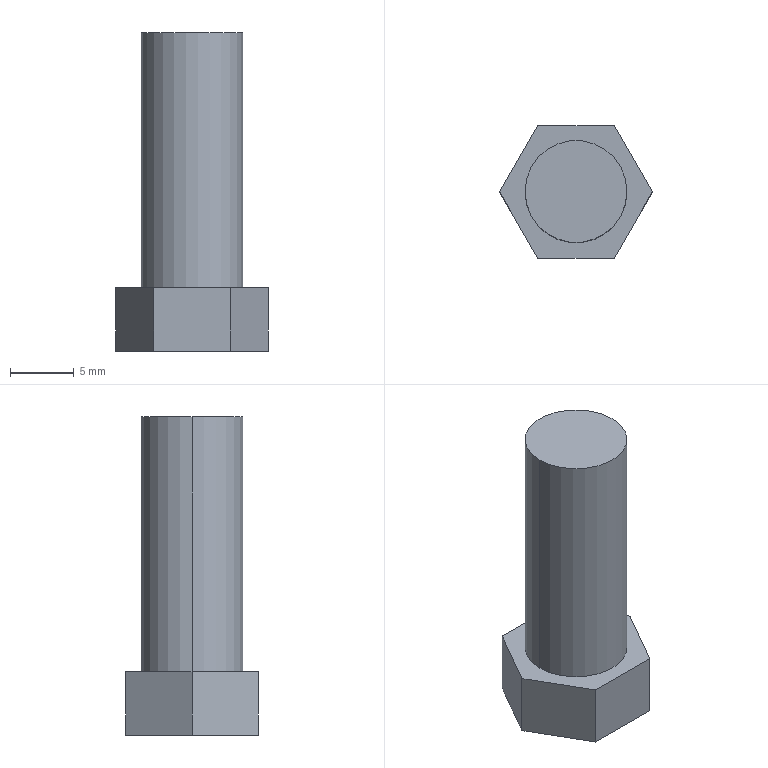Part | NX | features BREP 1, DATUM_CSYS 1, EXTRUDE 1, SKETCH 1 | 1 solid | 18 faces | box 12 x 10.392 x 25 mm | volume 1379 mm3 | plane 16 | cylinder 2 | commonest cylinder face diameters 8 x2
STEP:
#1=CARTESIAN_POINT('',(4.,0.,25.));
#2=VERTEX_POINT('',#1);
#3=CARTESIAN_POINT('',(-4.,0.,25.));
#4=VERTEX_POINT('',#3);
#5=CARTESIAN_POINT('',(0.,0.,25.));
#6=DIRECTION('',(0.,0.,1.));
#7=DIRECTION('',(1.,0.,0.));
#8=AXIS2_PLACEMENT_3D('',#5,#6,#7);
#9=CIRCLE('',#8,4.);
#10=EDGE_CURVE('',#2,#4,#9,.T.);
#11=ORIENTED_EDGE('',*,*,#10,.F.);
#12=CARTESIAN_POINT('',(4.,0.,5.));
#13=VERTEX_POINT('',#12);
#14=CARTESIAN_POINT('',(4.,0.,10.));
#15=DIRECTION('',(0.,0.,-1.));
#16=VECTOR('',#15,1000.);
#17=LINE('',#14,#16);
#18=EDGE_CURVE('',#13,#2,#17,.F.);
#19=ORIENTED_EDGE('',*,*,#18,.F.);
#20=CARTESIAN_POINT('',(-4.,0.,5.));
#21=VERTEX_POINT('',#20);
#22=CARTESIAN_POINT('',(0.,0.,5.));
#23=DIRECTION('',(0.,0.,1.));
#24=DIRECTION('',(1.,0.,0.));
#25=AXIS2_PLACEMENT_3D('',#22,#23,#24);
#26=CIRCLE('',#25,4.);
#27=EDGE_CURVE('',#13,#21,#26,.T.);
#28=ORIENTED_EDGE('',*,*,#27,.T.);
#29=CARTESIAN_POINT('',(-4.,0.,10.));
#30=DIRECTION('',(0.,0.,-1.));
#31=VECTOR('',#30,1000.);
#32=LINE('',#29,#31);
#33=EDGE_CURVE('',#21,#4,#32,.F.);
#34=ORIENTED_EDGE('',*,*,#33,.T.);
#35=EDGE_LOOP('',(#11,#19,#28,#34));
#36=FACE_BOUND('',#35,.T.);
#37=CARTESIAN_POINT('',(0.,0.,10.));
#38=DIRECTION('',(0.,0.,-1.));
#39=DIRECTION('',(1.,0.,0.));
#40=AXIS2_PLACEMENT_3D('',#37,#38,#39);
#41=CYLINDRICAL_SURFACE('',#40,4.);
#42=ADVANCED_FACE('',(#36),#41,.T.);
#43=CARTESIAN_POINT('',(3.,5.196,0.));
#44=VERTEX_POINT('',#43);
#45=CARTESIAN_POINT('',(-3.,5.196,0.));
#46=VERTEX_POINT('',#45);
#47=CARTESIAN_POINT('',(0.,5.196,0.));
#48=DIRECTION('',(-1.,0.,0.));
#49=VECTOR('',#48,1000.);
#50=LINE('',#47,#49);
#51=EDGE_CURVE('',#44,#46,#50,.T.);
#52=ORIENTED_EDGE('',*,*,#51,.T.);
#53=CARTESIAN_POINT('',(-3.,5.196,5.));
#54=VERTEX_POINT('',#53);
#55=CARTESIAN_POINT('',(-3.,5.196,5.));
#56=DIRECTION('',(0.,0.,-1.));
#57=VECTOR('',#56,1000.);
#58=LINE('',#55,#57);
#59=EDGE_CURVE('',#54,#46,#58,.T.);
#60=ORIENTED_EDGE('',*,*,#59,.F.);
#61=CARTESIAN_POINT('',(3.,5.196,5.));
#62=VERTEX_POINT('',#61);
#63=CARTESIAN_POINT('',(0.,5.196,5.));
#64=DIRECTION('',(-1.,0.,0.));
#65=VECTOR('',#64,1000.);
#66=LINE('',#63,#65);
#67=EDGE_CURVE('',#62,#54,#66,.T.);
#68=ORIENTED_EDGE('',*,*,#67,.F.);
#69=CARTESIAN_POINT('',(3.,5.196,5.));
#70=DIRECTION('',(0.,0.,-1.));
#71=VECTOR('',#70,1000.);
#72=LINE('',#69,#71);
#73=EDGE_CURVE('',#62,#44,#72,.T.);
#74=ORIENTED_EDGE('',*,*,#73,.T.);
#75=EDGE_LOOP('',(#52,#60,#68,#74));
#76=FACE_BOUND('',#75,.T.);
#77=CARTESIAN_POINT('',(0.,5.196,5.));
#78=DIRECTION('',(0.,-1.,0.));
#79=DIRECTION('',(-1.,0.,0.));
#80=AXIS2_PLACEMENT_3D('',#77,#78,#79);
#81=PLANE('',#80);
#82=ADVANCED_FACE('',(#76),#81,.F.);
#83=CARTESIAN_POINT('',(-6.,0.,0.));
#84=VERTEX_POINT('',#83);
#85=CARTESIAN_POINT('',(-4.5,2.598,0.));
#86=DIRECTION('',(-0.5,-0.866,0.));
#87=VECTOR('',#86,1000.);
#88=LINE('',#85,#87);
#89=EDGE_CURVE('',#46,#84,#88,.T.);
#90=ORIENTED_EDGE('',*,*,#89,.T.);
#91=CARTESIAN_POINT('',(-6.,0.,5.));
#92=VERTEX_POINT('',#91);
#93=CARTESIAN_POINT('',(-6.,0.,5.));
#94=DIRECTION('',(0.,0.,-1.));
#95=VECTOR('',#94,1000.);
#96=LINE('',#93,#95);
#97=EDGE_CURVE('',#92,#84,#96,.T.);
#98=ORIENTED_EDGE('',*,*,#97,.F.);
#99=CARTESIAN_POINT('',(-4.5,2.598,5.));
#100=DIRECTION('',(-0.5,-0.866,0.));
#101=VECTOR('',#100,1000.);
#102=LINE('',#99,#101);
#103=EDGE_CURVE('',#54,#92,#102,.T.);
#104=ORIENTED_EDGE('',*,*,#103,.F.);
#105=ORIENTED_EDGE('',*,*,#59,.T.);
#106=EDGE_LOOP('',(#90,#98,#104,#105));
#107=FACE_BOUND('',#106,.T.);
#108=CARTESIAN_POINT('',(-4.5,2.598,5.));
#109=DIRECTION('',(0.866,-0.5,0.));
#110=DIRECTION('',(-0.5,-0.866,0.));
#111=AXIS2_PLACEMENT_3D('',#108,#109,#110);
#112=PLANE('',#111);
#113=ADVANCED_FACE('',(#107),#112,.F.);
#114=CARTESIAN_POINT('',(-3.,-5.196,0.));
#115=VERTEX_POINT('',#114);
#116=CARTESIAN_POINT('',(-4.5,-2.598,0.));
#117=DIRECTION('',(0.5,-0.866,0.));
#118=VECTOR('',#117,1000.);
#119=LINE('',#116,#118);
#120=EDGE_CURVE('',#84,#115,#119,.T.);
#121=ORIENTED_EDGE('',*,*,#120,.T.);
#122=CARTESIAN_POINT('',(-3.,-5.196,5.));
#123=VERTEX_POINT('',#122);
#124=CARTESIAN_POINT('',(-3.,-5.196,5.));
#125=DIRECTION('',(0.,0.,-1.));
#126=VECTOR('',#125,1000.);
#127=LINE('',#124,#126);
#128=EDGE_CURVE('',#123,#115,#127,.T.);
#129=ORIENTED_EDGE('',*,*,#128,.F.);
#130=CARTESIAN_POINT('',(-4.5,-2.598,5.));
#131=DIRECTION('',(0.5,-0.866,0.));
#132=VECTOR('',#131,1000.);
#133=LINE('',#130,#132);
#134=EDGE_CURVE('',#92,#123,#133,.T.);
#135=ORIENTED_EDGE('',*,*,#134,.F.);
#136=ORIENTED_EDGE('',*,*,#97,.T.);
#137=EDGE_LOOP('',(#121,#129,#135,#136));
#138=FACE_BOUND('',#137,.T.);
#139=CARTESIAN_POINT('',(-4.5,-2.598,5.));
#140=DIRECTION('',(0.866,0.5,0.));
#141=DIRECTION('',(0.5,-0.866,0.));
#142=AXIS2_PLACEMENT_3D('',#139,#140,#141);
#143=PLANE('',#142);
#144=ADVANCED_FACE('',(#138),#143,.F.);
#145=CARTESIAN_POINT('',(3.,-5.196,0.));
#146=VERTEX_POINT('',#145);
#147=CARTESIAN_POINT('',(0.,-5.196,0.));
#148=DIRECTION('',(1.,0.,0.));
#149=VECTOR('',#148,1000.);
#150=LINE('',#147,#149);
#151=EDGE_CURVE('',#115,#146,#150,.T.);
#152=ORIENTED_EDGE('',*,*,#151,.T.);
#153=CARTESIAN_POINT('',(3.,-5.196,5.));
#154=VERTEX_POINT('',#153);
#155=CARTESIAN_POINT('',(3.,-5.196,5.));
#156=DIRECTION('',(0.,0.,-1.));
#157=VECTOR('',#156,1000.);
#158=LINE('',#155,#157);
#159=EDGE_CURVE('',#154,#146,#158,.T.);
#160=ORIENTED_EDGE('',*,*,#159,.F.);
#161=CARTESIAN_POINT('',(0.,-5.196,5.));
#162=DIRECTION('',(1.,0.,0.));
#163=VECTOR('',#162,1000.);
#164=LINE('',#161,#163);
#165=EDGE_CURVE('',#123,#154,#164,.T.);
#166=ORIENTED_EDGE('',*,*,#165,.F.);
#167=ORIENTED_EDGE('',*,*,#128,.T.);
#168=EDGE_LOOP('',(#152,#160,#166,#167));
#169=FACE_BOUND('',#168,.T.);
#170=CARTESIAN_POINT('',(0.,-5.196,5.));
#171=DIRECTION('',(0.,1.,0.));
#172=DIRECTION('',(1.,0.,0.));
#173=AXIS2_PLACEMENT_3D('',#170,#171,#172);
#174=PLANE('',#173);
#175=ADVANCED_FACE('',(#169),#174,.F.);
#176=CARTESIAN_POINT('',(6.,0.,0.));
#177=VERTEX_POINT('',#176);
#178=CARTESIAN_POINT('',(4.5,-2.598,0.));
#179=DIRECTION('',(0.5,0.866,0.));
#180=VECTOR('',#179,1000.);
#181=LINE('',#178,#180);
#182=EDGE_CURVE('',#146,#177,#181,.T.);
#183=ORIENTED_EDGE('',*,*,#182,.T.);
#184=CARTESIAN_POINT('',(6.,0.,5.));
#185=VERTEX_POINT('',#184);
#186=CARTESIAN_POINT('',(6.,0.,5.));
#187=DIRECTION('',(0.,0.,-1.));
#188=VECTOR('',#187,1000.);
#189=LINE('',#186,#188);
#190=EDGE_CURVE('',#185,#177,#189,.T.);
#191=ORIENTED_EDGE('',*,*,#190,.F.);
#192=CARTESIAN_POINT('',(4.5,-2.598,5.));
#193=DIRECTION('',(0.5,0.866,0.));
#194=VECTOR('',#193,1000.);
#195=LINE('',#192,#194);
#196=EDGE_CURVE('',#154,#185,#195,.T.);
#197=ORIENTED_EDGE('',*,*,#196,.F.);
#198=ORIENTED_EDGE('',*,*,#159,.T.);
#199=EDGE_LOOP('',(#183,#191,#197,#198));
#200=FACE_BOUND('',#199,.T.);
#201=CARTESIAN_POINT('',(4.5,-2.598,5.));
#202=DIRECTION('',(-0.866,0.5,0.));
#203=DIRECTION('',(0.5,0.866,0.));
#204=AXIS2_PLACEMENT_3D('',#201,#202,#203);
#205=PLANE('',#204);
#206=ADVANCED_FACE('',(#200),#205,.F.);
#207=CARTESIAN_POINT('',(4.5,2.598,0.));
#208=DIRECTION('',(-0.5,0.866,0.));
#209=VECTOR('',#208,1000.);
#210=LINE('',#207,#209);
#211=EDGE_CURVE('',#177,#44,#210,.T.);
#212=ORIENTED_EDGE('',*,*,#211,.T.);
#213=ORIENTED_EDGE('',*,*,#73,.F.);
#214=CARTESIAN_POINT('',(4.5,2.598,5.));
#215=DIRECTION('',(-0.5,0.866,0.));
#216=VECTOR('',#215,1000.);
#217=LINE('',#214,#216);
#218=EDGE_CURVE('',#185,#62,#217,.T.);
#219=ORIENTED_EDGE('',*,*,#218,.F.);
#220=ORIENTED_EDGE('',*,*,#190,.T.);
#221=EDGE_LOOP('',(#212,#213,#219,#220));
#222=FACE_BOUND('',#221,.T.);
#223=CARTESIAN_POINT('',(4.5,2.598,5.));
#224=DIRECTION('',(-0.866,-0.5,0.));
#225=DIRECTION('',(-0.5,0.866,0.));
#226=AXIS2_PLACEMENT_3D('',#223,#224,#225);
#227=PLANE('',#226);
#228=ADVANCED_FACE('',(#222),#227,.F.);
#229=CARTESIAN_POINT('',(0.,0.,5.));
#230=DIRECTION('',(0.,0.,1.));
#231=DIRECTION('',(1.,0.,0.));
#232=AXIS2_PLACEMENT_3D('',#229,#230,#231);
#233=CIRCLE('',#232,4.);
#234=EDGE_CURVE('',#21,#13,#233,.T.);
#235=ORIENTED_EDGE('',*,*,#234,.F.);
#236=ORIENTED_EDGE('',*,*,#27,.F.);
#237=EDGE_LOOP('',(#235,#236));
#238=FACE_BOUND('',#237,.T.);
#239=ORIENTED_EDGE('',*,*,#67,.T.);
#240=ORIENTED_EDGE('',*,*,#103,.T.);
#241=ORIENTED_EDGE('',*,*,#134,.T.);
#242=ORIENTED_EDGE('',*,*,#165,.T.);
#243=ORIENTED_EDGE('',*,*,#196,.T.);
#244=ORIENTED_EDGE('',*,*,#218,.T.);
#245=EDGE_LOOP('',(#239,#240,#241,#242,#243,#244));
#246=FACE_BOUND('',#245,.T.);
#247=CARTESIAN_POINT('',(0.,0.,5.));
#248=DIRECTION('',(0.,0.,1.));
#249=DIRECTION('',(-1.,0.,0.));
#250=AXIS2_PLACEMENT_3D('',#247,#248,#249);
#251=PLANE('',#250);
#252=ADVANCED_FACE('',(#238,#246),#251,.T.);
#253=CARTESIAN_POINT('',(-2.085,-2.767,0.));
#254=VERTEX_POINT('',#253);
#255=CARTESIAN_POINT('',(-3.438,0.4222,0.));
#256=VERTEX_POINT('',#255);
#257=CARTESIAN_POINT('',(-2.085,-2.767,0.));
#258=DIRECTION('',(-0.3907,0.9205,0.));
#259=VECTOR('',#258,1000.);
#260=LINE('',#257,#259);
#261=EDGE_CURVE('',#254,#256,#260,.T.);
#262=ORIENTED_EDGE('',*,*,#261,.F.);
#263=CARTESIAN_POINT('',(1.354,-3.189,0.));
#264=VERTEX_POINT('',#263);
#265=CARTESIAN_POINT('',(1.354,-3.189,0.));
#266=DIRECTION('',(-0.9925,0.1219,0.));
#267=VECTOR('',#266,1000.);
#268=LINE('',#265,#267);
#269=EDGE_CURVE('',#264,#254,#268,.T.);
#270=ORIENTED_EDGE('',*,*,#269,.F.);
#271=CARTESIAN_POINT('',(3.438,-0.4222,0.));
#272=VERTEX_POINT('',#271);
#273=CARTESIAN_POINT('',(3.438,-0.4222,0.));
#274=DIRECTION('',(-0.6018,-0.7986,0.));
#275=VECTOR('',#274,1000.);
#276=LINE('',#273,#275);
#277=EDGE_CURVE('',#272,#264,#276,.T.);
#278=ORIENTED_EDGE('',*,*,#277,.F.);
#279=CARTESIAN_POINT('',(2.085,2.767,0.));
#280=VERTEX_POINT('',#279);
#281=CARTESIAN_POINT('',(2.085,2.767,0.));
#282=DIRECTION('',(0.3907,-0.9205,0.));
#283=VECTOR('',#282,1000.);
#284=LINE('',#281,#283);
#285=EDGE_CURVE('',#280,#272,#284,.T.);
#286=ORIENTED_EDGE('',*,*,#285,.F.);
#287=CARTESIAN_POINT('',(-1.354,3.189,0.));
#288=VERTEX_POINT('',#287);
#289=CARTESIAN_POINT('',(-1.354,3.189,0.));
#290=DIRECTION('',(0.9925,-0.1219,0.));
#291=VECTOR('',#290,1000.);
#292=LINE('',#289,#291);
#293=EDGE_CURVE('',#288,#280,#292,.T.);
#294=ORIENTED_EDGE('',*,*,#293,.F.);
#295=CARTESIAN_POINT('',(-3.438,0.4222,0.));
#296=DIRECTION('',(0.6018,0.7986,0.));
#297=VECTOR('',#296,1000.);
#298=LINE('',#295,#297);
#299=EDGE_CURVE('',#256,#288,#298,.T.);
#300=ORIENTED_EDGE('',*,*,#299,.F.);
#301=EDGE_LOOP('',(#262,#270,#278,#286,#294,#300));
#302=FACE_BOUND('',#301,.T.);
#303=ORIENTED_EDGE('',*,*,#51,.F.);
#304=ORIENTED_EDGE('',*,*,#211,.F.);
#305=ORIENTED_EDGE('',*,*,#182,.F.);
#306=ORIENTED_EDGE('',*,*,#151,.F.);
#307=ORIENTED_EDGE('',*,*,#120,.F.);
#308=ORIENTED_EDGE('',*,*,#89,.F.);
#309=EDGE_LOOP('',(#303,#304,#305,#306,#307,#308));
#310=FACE_BOUND('',#309,.T.);
#311=CARTESIAN_POINT('',(0.,0.,0.));
#312=DIRECTION('',(0.,0.,1.));
#313=DIRECTION('',(-1.,0.,0.));
#314=AXIS2_PLACEMENT_3D('',#311,#312,#313);
#315=PLANE('',#314);
#316=ADVANCED_FACE('',(#302,#310),#315,.F.);
#317=ORIENTED_EDGE('',*,*,#18,.T.);
#318=CARTESIAN_POINT('',(0.,0.,25.));
#319=DIRECTION('',(0.,0.,1.));
#320=DIRECTION('',(1.,0.,0.));
#321=AXIS2_PLACEMENT_3D('',#318,#319,#320);
#322=CIRCLE('',#321,4.);
#323=EDGE_CURVE('',#4,#2,#322,.T.);
#324=ORIENTED_EDGE('',*,*,#323,.F.);
#325=ORIENTED_EDGE('',*,*,#33,.F.);
#326=ORIENTED_EDGE('',*,*,#234,.T.);
#327=EDGE_LOOP('',(#317,#324,#325,#326));
#328=FACE_BOUND('',#327,.T.);
#329=CARTESIAN_POINT('',(0.,0.,10.));
#330=DIRECTION('',(0.,0.,-1.));
#331=DIRECTION('',(1.,0.,0.));
#332=AXIS2_PLACEMENT_3D('',#329,#330,#331);
#333=CYLINDRICAL_SURFACE('',#332,4.);
#334=ADVANCED_FACE('',(#328),#333,.T.);
#335=ORIENTED_EDGE('',*,*,#323,.T.);
#336=ORIENTED_EDGE('',*,*,#10,.T.);
#337=EDGE_LOOP('',(#335,#336));
#338=FACE_BOUND('',#337,.T.);
#339=CARTESIAN_POINT('',(0.,0.,25.));
#340=DIRECTION('',(0.,0.,1.));
#341=DIRECTION('',(-1.,0.,0.));
#342=AXIS2_PLACEMENT_3D('',#339,#340,#341);
#343=PLANE('',#342);
#344=ADVANCED_FACE('',(#338),#343,.T.);
#345=ORIENTED_EDGE('',*,*,#269,.T.);
#346=CARTESIAN_POINT('',(-2.085,-2.767,3.));
#347=VERTEX_POINT('',#346);
#348=CARTESIAN_POINT('',(-2.085,-2.767,3.));
#349=DIRECTION('',(0.,0.,-1.));
#350=VECTOR('',#349,1000.);
#351=LINE('',#348,#350);
#352=EDGE_CURVE('',#254,#347,#351,.F.);
#353=ORIENTED_EDGE('',*,*,#352,.T.);
#354=CARTESIAN_POINT('',(1.354,-3.189,3.));
#355=VERTEX_POINT('',#354);
#356=CARTESIAN_POINT('',(1.354,-3.189,3.));
#357=DIRECTION('',(-0.9925,0.1219,0.));
#358=VECTOR('',#357,1000.);
#359=LINE('',#356,#358);
#360=EDGE_CURVE('',#347,#355,#359,.F.);
#361=ORIENTED_EDGE('',*,*,#360,.T.);
#362=CARTESIAN_POINT('',(1.354,-3.189,3.));
#363=DIRECTION('',(0.,0.,-1.));
#364=VECTOR('',#363,1000.);
#365=LINE('',#362,#364);
#366=EDGE_CURVE('',#264,#355,#365,.F.);
#367=ORIENTED_EDGE('',*,*,#366,.F.);
#368=EDGE_LOOP('',(#345,#353,#361,#367));
#369=FACE_BOUND('',#368,.T.);
#370=CARTESIAN_POINT('',(1.354,-3.189,3.));
#371=DIRECTION('',(-0.1219,-0.9925,0.));
#372=DIRECTION('',(0.9925,-0.1219,0.));
#373=AXIS2_PLACEMENT_3D('',#370,#371,#372);
#374=PLANE('',#373);
#375=ADVANCED_FACE('',(#369),#374,.F.);
#376=ORIENTED_EDGE('',*,*,#261,.T.);
#377=CARTESIAN_POINT('',(-3.438,0.4222,3.));
#378=VERTEX_POINT('',#377);
#379=CARTESIAN_POINT('',(-3.438,0.4222,3.));
#380=DIRECTION('',(0.,0.,-1.));
#381=VECTOR('',#380,1000.);
#382=LINE('',#379,#381);
#383=EDGE_CURVE('',#256,#378,#382,.F.);
#384=ORIENTED_EDGE('',*,*,#383,.T.);
#385=CARTESIAN_POINT('',(-2.085,-2.767,3.));
#386=DIRECTION('',(-0.3907,0.9205,0.));
#387=VECTOR('',#386,1000.);
#388=LINE('',#385,#387);
#389=EDGE_CURVE('',#378,#347,#388,.F.);
#390=ORIENTED_EDGE('',*,*,#389,.T.);
#391=ORIENTED_EDGE('',*,*,#352,.F.);
#392=EDGE_LOOP('',(#376,#384,#390,#391));
#393=FACE_BOUND('',#392,.T.);
#394=CARTESIAN_POINT('',(-2.085,-2.767,3.));
#395=DIRECTION('',(-0.9205,-0.3907,0.));
#396=DIRECTION('',(0.3907,-0.9205,0.));
#397=AXIS2_PLACEMENT_3D('',#394,#395,#396);
#398=PLANE('',#397);
#399=ADVANCED_FACE('',(#393),#398,.F.);
#400=ORIENTED_EDGE('',*,*,#299,.T.);
#401=CARTESIAN_POINT('',(-1.354,3.189,3.));
#402=VERTEX_POINT('',#401);
#403=CARTESIAN_POINT('',(-1.354,3.189,3.));
#404=DIRECTION('',(0.,0.,-1.));
#405=VECTOR('',#404,1000.);
#406=LINE('',#403,#405);
#407=EDGE_CURVE('',#288,#402,#406,.F.);
#408=ORIENTED_EDGE('',*,*,#407,.T.);
#409=CARTESIAN_POINT('',(-3.438,0.4222,3.));
#410=DIRECTION('',(0.6018,0.7986,0.));
#411=VECTOR('',#410,1000.);
#412=LINE('',#409,#411);
#413=EDGE_CURVE('',#402,#378,#412,.F.);
#414=ORIENTED_EDGE('',*,*,#413,.T.);
#415=ORIENTED_EDGE('',*,*,#383,.F.);
#416=EDGE_LOOP('',(#400,#408,#414,#415));
#417=FACE_BOUND('',#416,.T.);
#418=CARTESIAN_POINT('',(-3.438,0.4222,3.));
#419=DIRECTION('',(-0.7986,0.6018,0.));
#420=DIRECTION('',(-0.6018,-0.7986,0.));
#421=AXIS2_PLACEMENT_3D('',#418,#419,#420);
#422=PLANE('',#421);
#423=ADVANCED_FACE('',(#417),#422,.F.);
#424=ORIENTED_EDGE('',*,*,#293,.T.);
#425=CARTESIAN_POINT('',(2.085,2.767,3.));
#426=VERTEX_POINT('',#425);
#427=CARTESIAN_POINT('',(2.085,2.767,3.));
#428=DIRECTION('',(0.,0.,-1.));
#429=VECTOR('',#428,1000.);
#430=LINE('',#427,#429);
#431=EDGE_CURVE('',#280,#426,#430,.F.);
#432=ORIENTED_EDGE('',*,*,#431,.T.);
#433=CARTESIAN_POINT('',(-1.354,3.189,3.));
#434=DIRECTION('',(0.9925,-0.1219,0.));
#435=VECTOR('',#434,1000.);
#436=LINE('',#433,#435);
#437=EDGE_CURVE('',#426,#402,#436,.F.);
#438=ORIENTED_EDGE('',*,*,#437,.T.);
#439=ORIENTED_EDGE('',*,*,#407,.F.);
#440=EDGE_LOOP('',(#424,#432,#438,#439));
#441=FACE_BOUND('',#440,.T.);
#442=CARTESIAN_POINT('',(-1.354,3.189,3.));
#443=DIRECTION('',(0.1219,0.9925,0.));
#444=DIRECTION('',(-0.9925,0.1219,0.));
#445=AXIS2_PLACEMENT_3D('',#442,#443,#444);
#446=PLANE('',#445);
#447=ADVANCED_FACE('',(#441),#446,.F.);
#448=ORIENTED_EDGE('',*,*,#285,.T.);
#449=CARTESIAN_POINT('',(3.438,-0.4222,3.));
#450=VERTEX_POINT('',#449);
#451=CARTESIAN_POINT('',(3.438,-0.4222,3.));
#452=DIRECTION('',(0.,0.,-1.));
#453=VECTOR('',#452,1000.);
#454=LINE('',#451,#453);
#455=EDGE_CURVE('',#272,#450,#454,.F.);
#456=ORIENTED_EDGE('',*,*,#455,.T.);
#457=CARTESIAN_POINT('',(2.085,2.767,3.));
#458=DIRECTION('',(0.3907,-0.9205,0.));
#459=VECTOR('',#458,1000.);
#460=LINE('',#457,#459);
#461=EDGE_CURVE('',#450,#426,#460,.F.);
#462=ORIENTED_EDGE('',*,*,#461,.T.);
#463=ORIENTED_EDGE('',*,*,#431,.F.);
#464=EDGE_LOOP('',(#448,#456,#462,#463));
#465=FACE_BOUND('',#464,.T.);
#466=CARTESIAN_POINT('',(2.085,2.767,3.));
#467=DIRECTION('',(0.9205,0.3907,0.));
#468=DIRECTION('',(-0.3907,0.9205,0.));
#469=AXIS2_PLACEMENT_3D('',#466,#467,#468);
#470=PLANE('',#469);
#471=ADVANCED_FACE('',(#465),#470,.F.);
#472=ORIENTED_EDGE('',*,*,#277,.T.);
#473=ORIENTED_EDGE('',*,*,#366,.T.);
#474=CARTESIAN_POINT('',(3.438,-0.4222,3.));
#475=DIRECTION('',(-0.6018,-0.7986,0.));
#476=VECTOR('',#475,1000.);
#477=LINE('',#474,#476);
#478=EDGE_CURVE('',#355,#450,#477,.F.);
#479=ORIENTED_EDGE('',*,*,#478,.T.);
#480=ORIENTED_EDGE('',*,*,#455,.F.);
#481=EDGE_LOOP('',(#472,#473,#479,#480));
#482=FACE_BOUND('',#481,.T.);
#483=CARTESIAN_POINT('',(3.438,-0.4222,3.));
#484=DIRECTION('',(0.7986,-0.6018,0.));
#485=DIRECTION('',(0.6018,0.7986,0.));
#486=AXIS2_PLACEMENT_3D('',#483,#484,#485);
#487=PLANE('',#486);
#488=ADVANCED_FACE('',(#482),#487,.F.);
#489=ORIENTED_EDGE('',*,*,#360,.F.);
#490=ORIENTED_EDGE('',*,*,#389,.F.);
#491=ORIENTED_EDGE('',*,*,#413,.F.);
#492=ORIENTED_EDGE('',*,*,#437,.F.);
#493=ORIENTED_EDGE('',*,*,#461,.F.);
#494=ORIENTED_EDGE('',*,*,#478,.F.);
#495=EDGE_LOOP('',(#489,#490,#491,#492,#493,#494));
#496=FACE_BOUND('',#495,.T.);
#497=CARTESIAN_POINT('',(0.,0.,3.));
#498=DIRECTION('',(0.,0.,-1.));
#499=DIRECTION('',(-1.,0.,0.));
#500=AXIS2_PLACEMENT_3D('',#497,#498,#499);
#501=PLANE('',#500);
#502=ADVANCED_FACE('',(#496),#501,.T.);
#503=CLOSED_SHELL('',(#42,#82,#113,#144,#175,#206,#228,#252,#316,#334,#344,#375,#399,#423,#447,#471,#488,#502));
#504=MANIFOLD_SOLID_BREP('',#503);
#505=(LENGTH_UNIT()NAMED_UNIT(*)SI_UNIT(.MILLI.,.METRE.));
#506=UNCERTAINTY_MEASURE_WITH_UNIT(LENGTH_MEASURE(0.00001),#505,'','');
#507=(NAMED_UNIT(*)PLANE_ANGLE_UNIT()SI_UNIT($,.RADIAN.));
#508=(NAMED_UNIT(*)SI_UNIT($,.STERADIAN.)SOLID_ANGLE_UNIT());
#509=(GEOMETRIC_REPRESENTATION_CONTEXT(3)GLOBAL_UNCERTAINTY_ASSIGNED_CONTEXT((#506))GLOBAL_UNIT_ASSIGNED_CONTEXT((#505,#507,#508))REPRESENTATION_CONTEXT('',''));
#510=ADVANCED_BREP_SHAPE_REPRESENTATION('',(#504),#509);